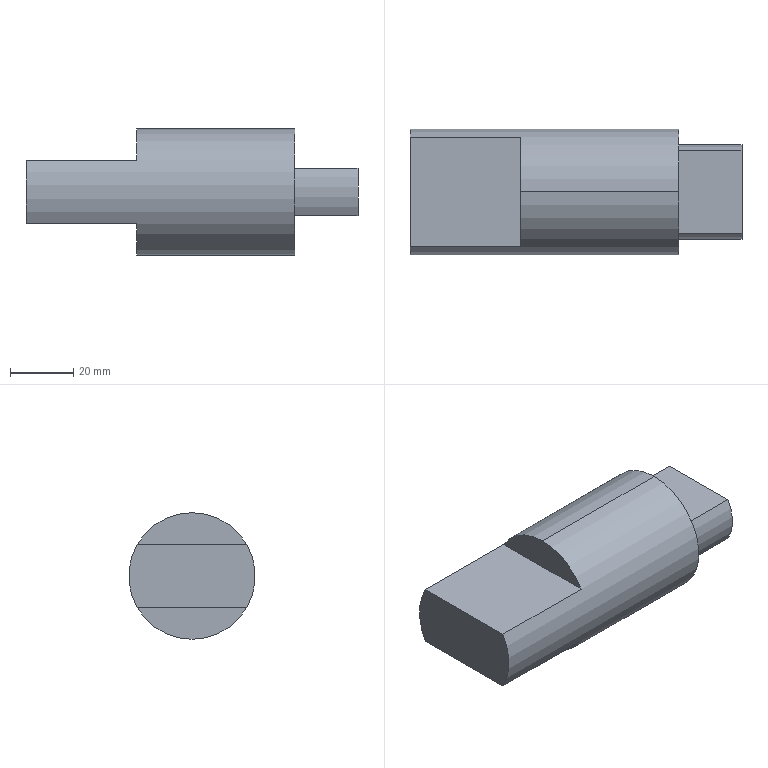Part | SolidWorks | 1 solid | 13 faces | box 105 x 40 x 40 mm | volume 98226 mm3 | plane 9 | cylinder 4 | commonest cylinder face diameters 30 x2 40 x2
STEP:
#1=CARTESIAN_POINT('',(-50.,0.,20.));
#2=VERTEX_POINT('',#1);
#3=CARTESIAN_POINT('',(-50.,17.321,10.));
#4=VERTEX_POINT('',#3);
#5=CARTESIAN_POINT('',(-50.,0.,0.));
#6=DIRECTION('',(-1.,0.,0.));
#7=DIRECTION('',(0.,0.,1.));
#8=AXIS2_PLACEMENT_3D('',#5,#6,#7);
#9=CIRCLE('',#8,20.);
#10=EDGE_CURVE('',#2,#4,#9,.T.);
#11=ORIENTED_EDGE('',*,*,#10,.F.);
#12=CARTESIAN_POINT('',(0.,0.,20.));
#13=VERTEX_POINT('',#12);
#14=CARTESIAN_POINT('',(-85.,0.,20.));
#15=DIRECTION('',(1.,0.,0.));
#16=VECTOR('',#15,1000.);
#17=LINE('',#14,#16);
#18=EDGE_CURVE('',#2,#13,#17,.T.);
#19=ORIENTED_EDGE('',*,*,#18,.T.);
#20=CARTESIAN_POINT('',(0.,0.,-20.));
#21=VERTEX_POINT('',#20);
#22=CARTESIAN_POINT('',(0.,0.,0.));
#23=DIRECTION('',(-1.,0.,0.));
#24=DIRECTION('',(0.,0.,1.));
#25=AXIS2_PLACEMENT_3D('',#22,#23,#24);
#26=CIRCLE('',#25,20.);
#27=EDGE_CURVE('',#13,#21,#26,.T.);
#28=ORIENTED_EDGE('',*,*,#27,.T.);
#29=CARTESIAN_POINT('',(-50.,0.,-20.));
#30=VERTEX_POINT('',#29);
#31=CARTESIAN_POINT('',(-85.,0.,-20.));
#32=DIRECTION('',(1.,0.,0.));
#33=VECTOR('',#32,1000.);
#34=LINE('',#31,#33);
#35=EDGE_CURVE('',#30,#21,#34,.T.);
#36=ORIENTED_EDGE('',*,*,#35,.F.);
#37=CARTESIAN_POINT('',(-50.,17.321,-10.));
#38=VERTEX_POINT('',#37);
#39=CARTESIAN_POINT('',(-50.,0.,0.));
#40=DIRECTION('',(-1.,0.,0.));
#41=DIRECTION('',(0.,0.,1.));
#42=AXIS2_PLACEMENT_3D('',#39,#40,#41);
#43=CIRCLE('',#42,20.);
#44=EDGE_CURVE('',#38,#30,#43,.T.);
#45=ORIENTED_EDGE('',*,*,#44,.F.);
#46=CARTESIAN_POINT('',(-85.,17.321,-10.));
#47=VERTEX_POINT('',#46);
#48=CARTESIAN_POINT('',(-50.,17.321,-10.));
#49=DIRECTION('',(-1.,0.,0.));
#50=VECTOR('',#49,1000.);
#51=LINE('',#48,#50);
#52=EDGE_CURVE('',#38,#47,#51,.T.);
#53=ORIENTED_EDGE('',*,*,#52,.T.);
#54=CARTESIAN_POINT('',(-85.,17.321,10.));
#55=VERTEX_POINT('',#54);
#56=CARTESIAN_POINT('',(-85.,0.,0.));
#57=DIRECTION('',(-1.,0.,0.));
#58=DIRECTION('',(0.,0.,1.));
#59=AXIS2_PLACEMENT_3D('',#56,#57,#58);
#60=CIRCLE('',#59,20.);
#61=EDGE_CURVE('',#55,#47,#60,.T.);
#62=ORIENTED_EDGE('',*,*,#61,.F.);
#63=CARTESIAN_POINT('',(-50.,17.321,10.));
#64=DIRECTION('',(-1.,0.,0.));
#65=VECTOR('',#64,1000.);
#66=LINE('',#63,#65);
#67=EDGE_CURVE('',#4,#55,#66,.T.);
#68=ORIENTED_EDGE('',*,*,#67,.F.);
#69=EDGE_LOOP('',(#11,#19,#28,#36,#45,#53,#62,#68));
#70=FACE_OUTER_BOUND('',#69,.T.);
#71=CARTESIAN_POINT('',(-85.,0.,0.));
#72=DIRECTION('',(1.,0.,0.));
#73=DIRECTION('',(0.,0.,-1.));
#74=AXIS2_PLACEMENT_3D('',#71,#72,#73);
#75=CYLINDRICAL_SURFACE('',#74,20.);
#76=ADVANCED_FACE('',(#70),#75,.T.);
#77=ORIENTED_EDGE('',*,*,#18,.F.);
#78=CARTESIAN_POINT('',(-50.,-17.321,10.));
#79=VERTEX_POINT('',#78);
#80=CARTESIAN_POINT('',(-50.,0.,0.));
#81=DIRECTION('',(-1.,0.,0.));
#82=DIRECTION('',(0.,0.,1.));
#83=AXIS2_PLACEMENT_3D('',#80,#81,#82);
#84=CIRCLE('',#83,20.);
#85=EDGE_CURVE('',#79,#2,#84,.T.);
#86=ORIENTED_EDGE('',*,*,#85,.F.);
#87=CARTESIAN_POINT('',(-85.,-17.321,10.));
#88=VERTEX_POINT('',#87);
#89=CARTESIAN_POINT('',(-50.,-17.321,10.));
#90=DIRECTION('',(-1.,0.,0.));
#91=VECTOR('',#90,1000.);
#92=LINE('',#89,#91);
#93=EDGE_CURVE('',#79,#88,#92,.T.);
#94=ORIENTED_EDGE('',*,*,#93,.T.);
#95=CARTESIAN_POINT('',(-85.,-17.321,-10.));
#96=VERTEX_POINT('',#95);
#97=CARTESIAN_POINT('',(-85.,0.,0.));
#98=DIRECTION('',(-1.,0.,0.));
#99=DIRECTION('',(0.,0.,1.));
#100=AXIS2_PLACEMENT_3D('',#97,#98,#99);
#101=CIRCLE('',#100,20.);
#102=EDGE_CURVE('',#96,#88,#101,.T.);
#103=ORIENTED_EDGE('',*,*,#102,.F.);
#104=CARTESIAN_POINT('',(-50.,-17.321,-10.));
#105=VERTEX_POINT('',#104);
#106=CARTESIAN_POINT('',(-50.,-17.321,-10.));
#107=DIRECTION('',(-1.,0.,0.));
#108=VECTOR('',#107,1000.);
#109=LINE('',#106,#108);
#110=EDGE_CURVE('',#105,#96,#109,.T.);
#111=ORIENTED_EDGE('',*,*,#110,.F.);
#112=CARTESIAN_POINT('',(-50.,0.,0.));
#113=DIRECTION('',(-1.,0.,0.));
#114=DIRECTION('',(0.,0.,1.));
#115=AXIS2_PLACEMENT_3D('',#112,#113,#114);
#116=CIRCLE('',#115,20.);
#117=EDGE_CURVE('',#30,#105,#116,.T.);
#118=ORIENTED_EDGE('',*,*,#117,.F.);
#119=ORIENTED_EDGE('',*,*,#35,.T.);
#120=CARTESIAN_POINT('',(0.,0.,0.));
#121=DIRECTION('',(-1.,0.,0.));
#122=DIRECTION('',(0.,0.,1.));
#123=AXIS2_PLACEMENT_3D('',#120,#121,#122);
#124=CIRCLE('',#123,20.);
#125=EDGE_CURVE('',#21,#13,#124,.T.);
#126=ORIENTED_EDGE('',*,*,#125,.T.);
#127=EDGE_LOOP('',(#77,#86,#94,#103,#111,#118,#119,#126));
#128=FACE_OUTER_BOUND('',#127,.T.);
#129=CARTESIAN_POINT('',(-85.,0.,0.));
#130=DIRECTION('',(1.,0.,0.));
#131=DIRECTION('',(0.,0.,-1.));
#132=AXIS2_PLACEMENT_3D('',#129,#130,#131);
#133=CYLINDRICAL_SURFACE('',#132,20.);
#134=ADVANCED_FACE('',(#128),#133,.T.);
#135=CARTESIAN_POINT('',(-85.,0.,10.));
#136=DIRECTION('',(0.,-1.,0.));
#137=VECTOR('',#136,1000.);
#138=LINE('',#135,#137);
#139=EDGE_CURVE('',#55,#88,#138,.T.);
#140=ORIENTED_EDGE('',*,*,#139,.F.);
#141=ORIENTED_EDGE('',*,*,#61,.T.);
#142=CARTESIAN_POINT('',(-85.,0.,-10.));
#143=DIRECTION('',(0.,-1.,0.));
#144=VECTOR('',#143,1000.);
#145=LINE('',#142,#144);
#146=EDGE_CURVE('',#47,#96,#145,.T.);
#147=ORIENTED_EDGE('',*,*,#146,.T.);
#148=ORIENTED_EDGE('',*,*,#102,.T.);
#149=EDGE_LOOP('',(#140,#141,#147,#148));
#150=FACE_OUTER_BOUND('',#149,.T.);
#151=CARTESIAN_POINT('',(-85.,0.,0.));
#152=DIRECTION('',(-1.,0.,0.));
#153=DIRECTION('',(0.,0.,1.));
#154=AXIS2_PLACEMENT_3D('',#151,#152,#153);
#155=PLANE('',#154);
#156=ADVANCED_FACE('',(#150),#155,.T.);
#157=CARTESIAN_POINT('',(0.,12.99,-7.5));
#158=VERTEX_POINT('',#157);
#159=CARTESIAN_POINT('',(0.,12.99,7.5));
#160=VERTEX_POINT('',#159);
#161=CARTESIAN_POINT('',(0.,0.,0.));
#162=DIRECTION('',(1.,0.,0.));
#163=DIRECTION('',(0.,0.,-1.));
#164=AXIS2_PLACEMENT_3D('',#161,#162,#163);
#165=CIRCLE('',#164,15.);
#166=EDGE_CURVE('',#158,#160,#165,.T.);
#167=ORIENTED_EDGE('',*,*,#166,.T.);
#168=CARTESIAN_POINT('',(20.,12.99,7.5));
#169=VERTEX_POINT('',#168);
#170=CARTESIAN_POINT('',(20.,12.99,7.5));
#171=DIRECTION('',(-1.,0.,0.));
#172=VECTOR('',#171,1000.);
#173=LINE('',#170,#172);
#174=EDGE_CURVE('',#169,#160,#173,.T.);
#175=ORIENTED_EDGE('',*,*,#174,.F.);
#176=CARTESIAN_POINT('',(20.,12.99,-7.5));
#177=VERTEX_POINT('',#176);
#178=CARTESIAN_POINT('',(20.,0.,0.));
#179=DIRECTION('',(1.,0.,0.));
#180=DIRECTION('',(0.,0.,-1.));
#181=AXIS2_PLACEMENT_3D('',#178,#179,#180);
#182=CIRCLE('',#181,15.);
#183=EDGE_CURVE('',#177,#169,#182,.T.);
#184=ORIENTED_EDGE('',*,*,#183,.F.);
#185=CARTESIAN_POINT('',(20.,12.99,-7.5));
#186=DIRECTION('',(-1.,0.,0.));
#187=VECTOR('',#186,1000.);
#188=LINE('',#185,#187);
#189=EDGE_CURVE('',#177,#158,#188,.T.);
#190=ORIENTED_EDGE('',*,*,#189,.T.);
#191=EDGE_LOOP('',(#167,#175,#184,#190));
#192=FACE_OUTER_BOUND('',#191,.T.);
#193=CARTESIAN_POINT('',(20.,0.,0.));
#194=DIRECTION('',(-1.,0.,0.));
#195=DIRECTION('',(0.,0.,1.));
#196=AXIS2_PLACEMENT_3D('',#193,#194,#195);
#197=CYLINDRICAL_SURFACE('',#196,15.);
#198=ADVANCED_FACE('',(#192),#197,.T.);
#199=CARTESIAN_POINT('',(0.,-12.99,7.5));
#200=VERTEX_POINT('',#199);
#201=CARTESIAN_POINT('',(0.,0.,7.5));
#202=DIRECTION('',(0.,-1.,0.));
#203=VECTOR('',#202,1000.);
#204=LINE('',#201,#203);
#205=EDGE_CURVE('',#160,#200,#204,.T.);
#206=ORIENTED_EDGE('',*,*,#205,.T.);
#207=CARTESIAN_POINT('',(20.,-12.99,7.5));
#208=VERTEX_POINT('',#207);
#209=CARTESIAN_POINT('',(20.,-12.99,7.5));
#210=DIRECTION('',(-1.,0.,0.));
#211=VECTOR('',#210,1000.);
#212=LINE('',#209,#211);
#213=EDGE_CURVE('',#208,#200,#212,.T.);
#214=ORIENTED_EDGE('',*,*,#213,.F.);
#215=CARTESIAN_POINT('',(20.,0.,7.5));
#216=DIRECTION('',(0.,-1.,0.));
#217=VECTOR('',#216,1000.);
#218=LINE('',#215,#217);
#219=EDGE_CURVE('',#169,#208,#218,.T.);
#220=ORIENTED_EDGE('',*,*,#219,.F.);
#221=ORIENTED_EDGE('',*,*,#174,.T.);
#222=EDGE_LOOP('',(#206,#214,#220,#221));
#223=FACE_OUTER_BOUND('',#222,.T.);
#224=CARTESIAN_POINT('',(20.,0.,7.5));
#225=DIRECTION('',(0.,0.,-1.));
#226=DIRECTION('',(-1.,0.,0.));
#227=AXIS2_PLACEMENT_3D('',#224,#225,#226);
#228=PLANE('',#227);
#229=ADVANCED_FACE('',(#223),#228,.F.);
#230=CARTESIAN_POINT('',(0.,-12.99,-7.5));
#231=VERTEX_POINT('',#230);
#232=CARTESIAN_POINT('',(0.,0.,0.));
#233=DIRECTION('',(1.,0.,0.));
#234=DIRECTION('',(0.,0.,-1.));
#235=AXIS2_PLACEMENT_3D('',#232,#233,#234);
#236=CIRCLE('',#235,15.);
#237=EDGE_CURVE('',#200,#231,#236,.T.);
#238=ORIENTED_EDGE('',*,*,#237,.T.);
#239=CARTESIAN_POINT('',(20.,-12.99,-7.5));
#240=VERTEX_POINT('',#239);
#241=CARTESIAN_POINT('',(20.,-12.99,-7.5));
#242=DIRECTION('',(-1.,0.,0.));
#243=VECTOR('',#242,1000.);
#244=LINE('',#241,#243);
#245=EDGE_CURVE('',#240,#231,#244,.T.);
#246=ORIENTED_EDGE('',*,*,#245,.F.);
#247=CARTESIAN_POINT('',(20.,0.,0.));
#248=DIRECTION('',(1.,0.,0.));
#249=DIRECTION('',(0.,0.,-1.));
#250=AXIS2_PLACEMENT_3D('',#247,#248,#249);
#251=CIRCLE('',#250,15.);
#252=EDGE_CURVE('',#208,#240,#251,.T.);
#253=ORIENTED_EDGE('',*,*,#252,.F.);
#254=ORIENTED_EDGE('',*,*,#213,.T.);
#255=EDGE_LOOP('',(#238,#246,#253,#254));
#256=FACE_OUTER_BOUND('',#255,.T.);
#257=CARTESIAN_POINT('',(20.,0.,0.));
#258=DIRECTION('',(-1.,0.,0.));
#259=DIRECTION('',(0.,0.,1.));
#260=AXIS2_PLACEMENT_3D('',#257,#258,#259);
#261=CYLINDRICAL_SURFACE('',#260,15.);
#262=ADVANCED_FACE('',(#256),#261,.T.);
#263=CARTESIAN_POINT('',(0.,0.,-7.5));
#264=DIRECTION('',(0.,-1.,0.));
#265=VECTOR('',#264,1000.);
#266=LINE('',#263,#265);
#267=EDGE_CURVE('',#158,#231,#266,.T.);
#268=ORIENTED_EDGE('',*,*,#267,.F.);
#269=ORIENTED_EDGE('',*,*,#189,.F.);
#270=CARTESIAN_POINT('',(20.,0.,-7.5));
#271=DIRECTION('',(0.,-1.,0.));
#272=VECTOR('',#271,1000.);
#273=LINE('',#270,#272);
#274=EDGE_CURVE('',#177,#240,#273,.T.);
#275=ORIENTED_EDGE('',*,*,#274,.T.);
#276=ORIENTED_EDGE('',*,*,#245,.T.);
#277=EDGE_LOOP('',(#268,#269,#275,#276));
#278=FACE_OUTER_BOUND('',#277,.T.);
#279=CARTESIAN_POINT('',(20.,0.,-7.5));
#280=DIRECTION('',(0.,0.,-1.));
#281=DIRECTION('',(-1.,0.,0.));
#282=AXIS2_PLACEMENT_3D('',#279,#280,#281);
#283=PLANE('',#282);
#284=ADVANCED_FACE('',(#278),#283,.T.);
#285=ORIENTED_EDGE('',*,*,#183,.T.);
#286=ORIENTED_EDGE('',*,*,#219,.T.);
#287=ORIENTED_EDGE('',*,*,#252,.T.);
#288=ORIENTED_EDGE('',*,*,#274,.F.);
#289=EDGE_LOOP('',(#285,#286,#287,#288));
#290=FACE_OUTER_BOUND('',#289,.T.);
#291=CARTESIAN_POINT('',(20.,0.,0.));
#292=DIRECTION('',(1.,0.,0.));
#293=DIRECTION('',(0.,0.,-1.));
#294=AXIS2_PLACEMENT_3D('',#291,#292,#293);
#295=PLANE('',#294);
#296=ADVANCED_FACE('',(#290),#295,.T.);
#297=ORIENTED_EDGE('',*,*,#166,.F.);
#298=ORIENTED_EDGE('',*,*,#267,.T.);
#299=ORIENTED_EDGE('',*,*,#237,.F.);
#300=ORIENTED_EDGE('',*,*,#205,.F.);
#301=EDGE_LOOP('',(#297,#298,#299,#300));
#302=FACE_BOUND('',#301,.T.);
#303=ORIENTED_EDGE('',*,*,#125,.F.);
#304=ORIENTED_EDGE('',*,*,#27,.F.);
#305=EDGE_LOOP('',(#303,#304));
#306=FACE_OUTER_BOUND('',#305,.T.);
#307=CARTESIAN_POINT('',(0.,0.,0.));
#308=DIRECTION('',(-1.,0.,0.));
#309=DIRECTION('',(0.,0.,1.));
#310=AXIS2_PLACEMENT_3D('',#307,#308,#309);
#311=PLANE('',#310);
#312=ADVANCED_FACE('',(#302,#306),#311,.F.);
#313=ORIENTED_EDGE('',*,*,#146,.F.);
#314=ORIENTED_EDGE('',*,*,#52,.F.);
#315=CARTESIAN_POINT('',(-50.,0.,-10.));
#316=DIRECTION('',(0.,-1.,0.));
#317=VECTOR('',#316,1000.);
#318=LINE('',#315,#317);
#319=EDGE_CURVE('',#38,#105,#318,.T.);
#320=ORIENTED_EDGE('',*,*,#319,.T.);
#321=ORIENTED_EDGE('',*,*,#110,.T.);
#322=EDGE_LOOP('',(#313,#314,#320,#321));
#323=FACE_OUTER_BOUND('',#322,.T.);
#324=CARTESIAN_POINT('',(-50.,0.,-10.));
#325=DIRECTION('',(0.,0.,-1.));
#326=DIRECTION('',(-1.,0.,0.));
#327=AXIS2_PLACEMENT_3D('',#324,#325,#326);
#328=PLANE('',#327);
#329=ADVANCED_FACE('',(#323),#328,.T.);
#330=ORIENTED_EDGE('',*,*,#319,.F.);
#331=ORIENTED_EDGE('',*,*,#44,.T.);
#332=ORIENTED_EDGE('',*,*,#117,.T.);
#333=EDGE_LOOP('',(#330,#331,#332));
#334=FACE_OUTER_BOUND('',#333,.T.);
#335=CARTESIAN_POINT('',(-50.,0.,0.));
#336=DIRECTION('',(-1.,0.,0.));
#337=DIRECTION('',(0.,0.,1.));
#338=AXIS2_PLACEMENT_3D('',#335,#336,#337);
#339=PLANE('',#338);
#340=ADVANCED_FACE('',(#334),#339,.T.);
#341=ORIENTED_EDGE('',*,*,#139,.T.);
#342=ORIENTED_EDGE('',*,*,#93,.F.);
#343=CARTESIAN_POINT('',(-50.,0.,10.));
#344=DIRECTION('',(0.,-1.,0.));
#345=VECTOR('',#344,1000.);
#346=LINE('',#343,#345);
#347=EDGE_CURVE('',#4,#79,#346,.T.);
#348=ORIENTED_EDGE('',*,*,#347,.F.);
#349=ORIENTED_EDGE('',*,*,#67,.T.);
#350=EDGE_LOOP('',(#341,#342,#348,#349));
#351=FACE_OUTER_BOUND('',#350,.T.);
#352=CARTESIAN_POINT('',(-50.,0.,10.));
#353=DIRECTION('',(0.,0.,-1.));
#354=DIRECTION('',(-1.,0.,0.));
#355=AXIS2_PLACEMENT_3D('',#352,#353,#354);
#356=PLANE('',#355);
#357=ADVANCED_FACE('',(#351),#356,.F.);
#358=ORIENTED_EDGE('',*,*,#85,.T.);
#359=ORIENTED_EDGE('',*,*,#10,.T.);
#360=ORIENTED_EDGE('',*,*,#347,.T.);
#361=EDGE_LOOP('',(#358,#359,#360));
#362=FACE_OUTER_BOUND('',#361,.T.);
#363=CARTESIAN_POINT('',(-50.,0.,0.));
#364=DIRECTION('',(-1.,0.,0.));
#365=DIRECTION('',(0.,0.,1.));
#366=AXIS2_PLACEMENT_3D('',#363,#364,#365);
#367=PLANE('',#366);
#368=ADVANCED_FACE('',(#362),#367,.T.);
#369=CLOSED_SHELL('',(#76,#134,#156,#198,#229,#262,#284,#296,#312,#329,#340,#357,#368));
#370=MANIFOLD_SOLID_BREP('',#369);
#371=CARTESIAN_POINT('',(0.,0.,0.));
#372=DIRECTION('',(0.,0.,1.));
#373=DIRECTION('',(1.,0.,0.));
#374=AXIS2_PLACEMENT_3D('',#371,#372,#373);
#375=(LENGTH_UNIT()NAMED_UNIT(*)SI_UNIT(.MILLI.,.METRE.));
#376=UNCERTAINTY_MEASURE_WITH_UNIT(LENGTH_MEASURE(0.00001),#375,'','');
#377=(NAMED_UNIT(*)PLANE_ANGLE_UNIT()SI_UNIT($,.RADIAN.));
#378=(NAMED_UNIT(*)SI_UNIT($,.STERADIAN.)SOLID_ANGLE_UNIT());
#379=(GEOMETRIC_REPRESENTATION_CONTEXT(3)GLOBAL_UNCERTAINTY_ASSIGNED_CONTEXT((#376))GLOBAL_UNIT_ASSIGNED_CONTEXT((#375,#377,#378))REPRESENTATION_CONTEXT('',''));
#380=ADVANCED_BREP_SHAPE_REPRESENTATION('',(#370,#374),#379);